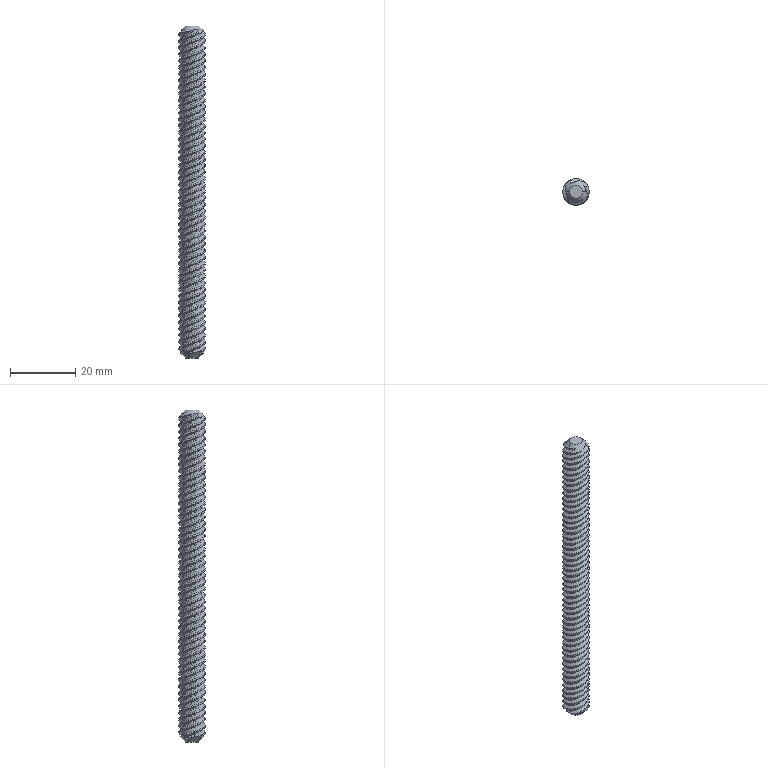Part | SolidWorks | features Helix 4, Sweep 4, RevCut 2, Extrusion 1, ICE 1 | 1 solid | 122 faces | box 8 x 8 x 101.6 mm | volume 3914 mm3 | cylinder 104 | spline 12 | cone 4 | plane 2 | commonest cylinder face diameters 6 x104